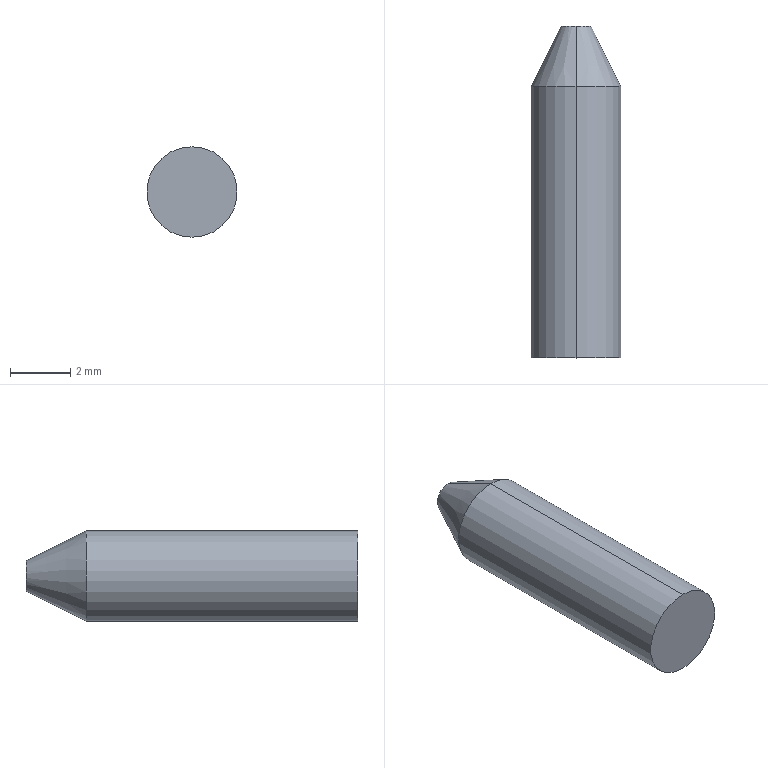Part | STEP file | 07-11 locating pin | 1 solid | 6 faces | box 3 x 11 x 3 mm | volume 70.424 mm3 | cone 2 | cylinder 2 | plane 2 | commonest cylinder face diameters 3 x2
STEP:
#1=CARTESIAN_POINT('',(0.,11.,0.5));
#2=VERTEX_POINT('',#1);
#3=CARTESIAN_POINT('',(0.,11.,-0.5));
#4=VERTEX_POINT('',#3);
#5=CARTESIAN_POINT('',(0.,11.,0.));
#6=DIRECTION('',(0.,1.,0.));
#7=DIRECTION('',(0.,0.,1.));
#8=AXIS2_PLACEMENT_3D('',#5,#6,#7);
#9=CIRCLE('',#8,0.5);
#10=EDGE_CURVE('',#2,#4,#9,.T.);
#11=ORIENTED_EDGE('',*,*,#10,.F.);
#12=CARTESIAN_POINT('',(0.,9.,1.5));
#13=VERTEX_POINT('',#12);
#14=CARTESIAN_POINT('',(0.,11.,0.5));
#15=DIRECTION('',(0.,-0.8944,0.4472));
#16=VECTOR('',#15,1000.);
#17=LINE('',#14,#16);
#18=EDGE_CURVE('',#2,#13,#17,.T.);
#19=ORIENTED_EDGE('',*,*,#18,.T.);
#20=CARTESIAN_POINT('',(0.,9.,-1.5));
#21=VERTEX_POINT('',#20);
#22=CARTESIAN_POINT('',(0.,9.,0.));
#23=DIRECTION('',(0.,-1.,0.));
#24=DIRECTION('',(0.,0.,1.));
#25=AXIS2_PLACEMENT_3D('',#22,#23,#24);
#26=CIRCLE('',#25,1.5);
#27=EDGE_CURVE('',#21,#13,#26,.T.);
#28=ORIENTED_EDGE('',*,*,#27,.F.);
#29=CARTESIAN_POINT('',(0.,11.,-0.5));
#30=DIRECTION('',(0.,-0.8944,-0.4472));
#31=VECTOR('',#30,1000.);
#32=LINE('',#29,#31);
#33=EDGE_CURVE('',#4,#21,#32,.T.);
#34=ORIENTED_EDGE('',*,*,#33,.F.);
#35=EDGE_LOOP('',(#11,#19,#28,#34));
#36=FACE_OUTER_BOUND('',#35,.T.);
#37=CARTESIAN_POINT('',(0.,11.,0.));
#38=DIRECTION('',(0.,-1.,0.));
#39=DIRECTION('',(0.,0.,-1.));
#40=AXIS2_PLACEMENT_3D('',#37,#38,#39);
#41=CONICAL_SURFACE('',#40,0.5,0.4636);
#42=ADVANCED_FACE('',(#36),#41,.T.);
#43=ORIENTED_EDGE('',*,*,#27,.T.);
#44=CARTESIAN_POINT('',(0.,0.,1.5));
#45=VERTEX_POINT('',#44);
#46=CARTESIAN_POINT('',(0.,11.,1.5));
#47=DIRECTION('',(0.,-1.,0.));
#48=VECTOR('',#47,1000.);
#49=LINE('',#46,#48);
#50=EDGE_CURVE('',#13,#45,#49,.T.);
#51=ORIENTED_EDGE('',*,*,#50,.T.);
#52=CARTESIAN_POINT('',(0.,0.,-1.5));
#53=VERTEX_POINT('',#52);
#54=CARTESIAN_POINT('',(0.,0.,0.));
#55=DIRECTION('',(0.,1.,0.));
#56=DIRECTION('',(0.,0.,1.));
#57=AXIS2_PLACEMENT_3D('',#54,#55,#56);
#58=CIRCLE('',#57,1.5);
#59=EDGE_CURVE('',#45,#53,#58,.T.);
#60=ORIENTED_EDGE('',*,*,#59,.T.);
#61=CARTESIAN_POINT('',(0.,11.,-1.5));
#62=DIRECTION('',(0.,-1.,0.));
#63=VECTOR('',#62,1000.);
#64=LINE('',#61,#63);
#65=EDGE_CURVE('',#21,#53,#64,.T.);
#66=ORIENTED_EDGE('',*,*,#65,.F.);
#67=EDGE_LOOP('',(#43,#51,#60,#66));
#68=FACE_OUTER_BOUND('',#67,.T.);
#69=CARTESIAN_POINT('',(0.,11.,0.));
#70=DIRECTION('',(0.,-1.,0.));
#71=DIRECTION('',(0.,0.,-1.));
#72=AXIS2_PLACEMENT_3D('',#69,#70,#71);
#73=CYLINDRICAL_SURFACE('',#72,1.5);
#74=ADVANCED_FACE('',(#68),#73,.T.);
#75=ORIENTED_EDGE('',*,*,#50,.F.);
#76=CARTESIAN_POINT('',(0.,9.,0.));
#77=DIRECTION('',(0.,-1.,0.));
#78=DIRECTION('',(0.,0.,1.));
#79=AXIS2_PLACEMENT_3D('',#76,#77,#78);
#80=CIRCLE('',#79,1.5);
#81=EDGE_CURVE('',#13,#21,#80,.T.);
#82=ORIENTED_EDGE('',*,*,#81,.T.);
#83=ORIENTED_EDGE('',*,*,#65,.T.);
#84=CARTESIAN_POINT('',(0.,0.,0.));
#85=DIRECTION('',(0.,1.,0.));
#86=DIRECTION('',(0.,0.,1.));
#87=AXIS2_PLACEMENT_3D('',#84,#85,#86);
#88=CIRCLE('',#87,1.5);
#89=EDGE_CURVE('',#53,#45,#88,.T.);
#90=ORIENTED_EDGE('',*,*,#89,.T.);
#91=EDGE_LOOP('',(#75,#82,#83,#90));
#92=FACE_OUTER_BOUND('',#91,.T.);
#93=CARTESIAN_POINT('',(0.,11.,0.));
#94=DIRECTION('',(0.,-1.,0.));
#95=DIRECTION('',(0.,0.,-1.));
#96=AXIS2_PLACEMENT_3D('',#93,#94,#95);
#97=CYLINDRICAL_SURFACE('',#96,1.5);
#98=ADVANCED_FACE('',(#92),#97,.T.);
#99=CARTESIAN_POINT('',(0.,11.,0.));
#100=DIRECTION('',(0.,1.,0.));
#101=DIRECTION('',(0.,0.,1.));
#102=AXIS2_PLACEMENT_3D('',#99,#100,#101);
#103=CIRCLE('',#102,0.5);
#104=EDGE_CURVE('',#4,#2,#103,.T.);
#105=ORIENTED_EDGE('',*,*,#104,.T.);
#106=ORIENTED_EDGE('',*,*,#10,.T.);
#107=EDGE_LOOP('',(#105,#106));
#108=FACE_OUTER_BOUND('',#107,.T.);
#109=CARTESIAN_POINT('',(0.,11.,0.));
#110=DIRECTION('',(0.,1.,0.));
#111=DIRECTION('',(0.,0.,1.));
#112=AXIS2_PLACEMENT_3D('',#109,#110,#111);
#113=PLANE('',#112);
#114=ADVANCED_FACE('',(#108),#113,.T.);
#115=ORIENTED_EDGE('',*,*,#89,.F.);
#116=ORIENTED_EDGE('',*,*,#59,.F.);
#117=EDGE_LOOP('',(#115,#116));
#118=FACE_OUTER_BOUND('',#117,.T.);
#119=CARTESIAN_POINT('',(0.,0.,0.));
#120=DIRECTION('',(0.,1.,0.));
#121=DIRECTION('',(0.,0.,1.));
#122=AXIS2_PLACEMENT_3D('',#119,#120,#121);
#123=PLANE('',#122);
#124=ADVANCED_FACE('',(#118),#123,.F.);
#125=ORIENTED_EDGE('',*,*,#18,.F.);
#126=ORIENTED_EDGE('',*,*,#104,.F.);
#127=ORIENTED_EDGE('',*,*,#33,.T.);
#128=ORIENTED_EDGE('',*,*,#81,.F.);
#129=EDGE_LOOP('',(#125,#126,#127,#128));
#130=FACE_OUTER_BOUND('',#129,.T.);
#131=CARTESIAN_POINT('',(0.,11.,0.));
#132=DIRECTION('',(0.,-1.,0.));
#133=DIRECTION('',(0.,0.,-1.));
#134=AXIS2_PLACEMENT_3D('',#131,#132,#133);
#135=CONICAL_SURFACE('',#134,0.5,0.4636);
#136=ADVANCED_FACE('',(#130),#135,.T.);
#137=CLOSED_SHELL('',(#42,#74,#98,#114,#124,#136));
#138=MANIFOLD_SOLID_BREP('',#137);
#139=CARTESIAN_POINT('',(0.,0.,0.));
#140=DIRECTION('',(0.,0.,1.));
#141=DIRECTION('',(1.,0.,0.));
#142=AXIS2_PLACEMENT_3D('',#139,#140,#141);
#143=(LENGTH_UNIT()NAMED_UNIT(*)SI_UNIT(.MILLI.,.METRE.));
#144=UNCERTAINTY_MEASURE_WITH_UNIT(LENGTH_MEASURE(0.00001),#143,'','');
#145=(NAMED_UNIT(*)PLANE_ANGLE_UNIT()SI_UNIT($,.RADIAN.));
#146=(NAMED_UNIT(*)SI_UNIT($,.STERADIAN.)SOLID_ANGLE_UNIT());
#147=(GEOMETRIC_REPRESENTATION_CONTEXT(3)GLOBAL_UNCERTAINTY_ASSIGNED_CONTEXT((#144))GLOBAL_UNIT_ASSIGNED_CONTEXT((#143,#145,#146))REPRESENTATION_CONTEXT('',''));
#148=ADVANCED_BREP_SHAPE_REPRESENTATION('',(#138,#142),#147);